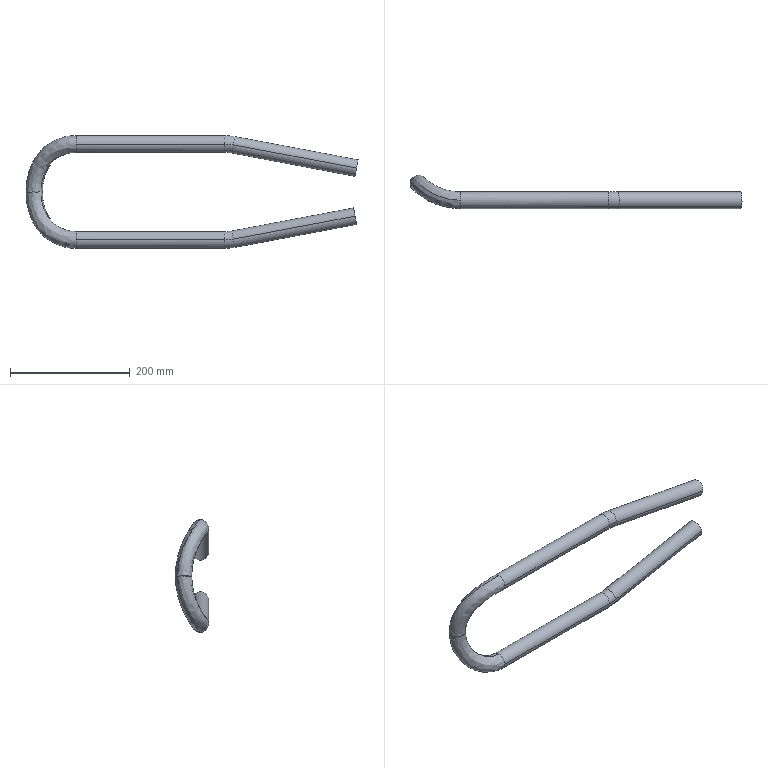Part | STEP file | PRT0001_68_13 | 1 solid | 34 faces | box 553.703 x 55.695 x 188 mm | volume 147514 mm3 | cylinder 16 | torus 8 | spline 8 | plane 2 | commonest cylinder face diameters 25 x8 28 x8